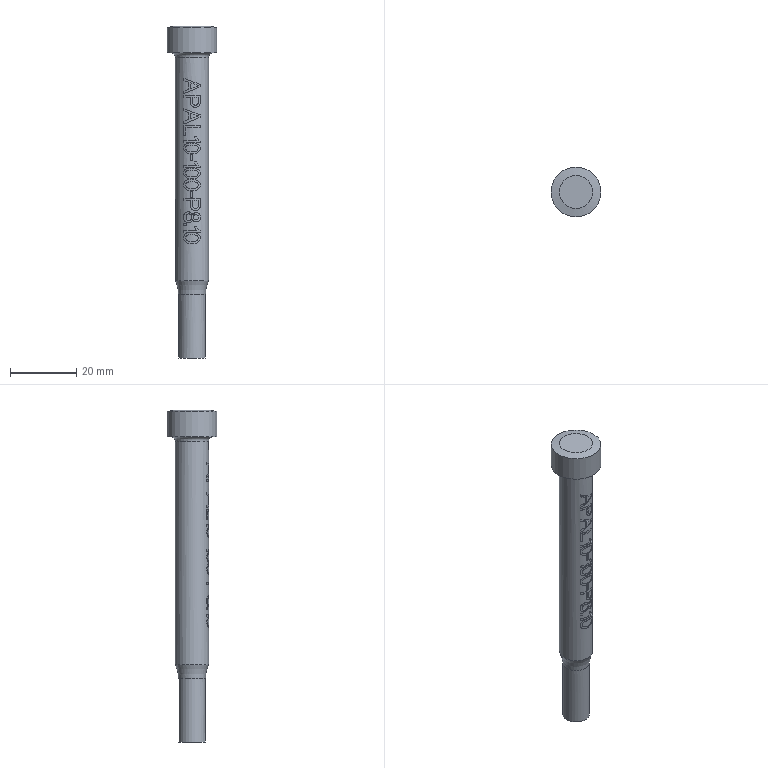Part | STEP file | PN_0050_id1066_x_t | 1 solid | 194 faces | box 15 x 15 x 100 mm | volume 8031 mm3 | plane 112 | cylinder 79 | torus 2 | cone 1 | commonest cylinder face diameters 9.8 x16 10 x11 2.089 x4 2.493 x4 2.5 x4 2.529 x4